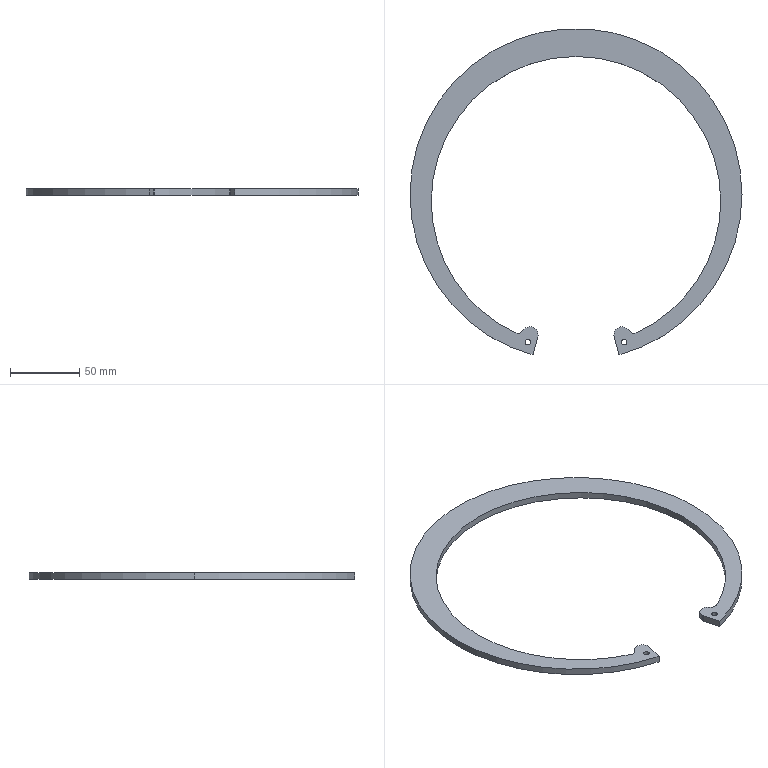Part | SolidWorks | features Extrusion 1 | 1 solid | 19 faces | box 240.5 x 236.403 x 4.75 mm | volume 49385 mm3 | cylinder 15 | plane 4 | commonest cylinder face diameters 4 x4 12 x3 209.7 x3 240.5 x3 8 x2
STEP:
#1=CARTESIAN_POINT('',(32.871,-106.959,2.375));
#2=VERTEX_POINT('',#1);
#3=CARTESIAN_POINT('',(36.871,-106.959,2.375));
#4=VERTEX_POINT('',#3);
#5=CARTESIAN_POINT('',(34.871,-106.959,2.375));
#6=DIRECTION('',(0.,0.,1.));
#7=DIRECTION('',(-1.,0.,0.));
#8=AXIS2_PLACEMENT_3D('',#5,#6,#7);
#9=CIRCLE('',#8,2.);
#10=EDGE_CURVE('',#2,#4,#9,.T.);
#11=ORIENTED_EDGE('',*,*,#10,.T.);
#12=CARTESIAN_POINT('',(36.871,-106.959,-2.375));
#13=VERTEX_POINT('',#12);
#14=CARTESIAN_POINT('',(36.871,-106.959,2.375));
#15=DIRECTION('',(0.,0.,-1.));
#16=VECTOR('',#15,1000.);
#17=LINE('',#14,#16);
#18=EDGE_CURVE('',#4,#13,#17,.T.);
#19=ORIENTED_EDGE('',*,*,#18,.T.);
#20=CARTESIAN_POINT('',(32.871,-106.959,-2.375));
#21=VERTEX_POINT('',#20);
#22=CARTESIAN_POINT('',(34.871,-106.959,-2.375));
#23=DIRECTION('',(0.,0.,1.));
#24=DIRECTION('',(-1.,0.,0.));
#25=AXIS2_PLACEMENT_3D('',#22,#23,#24);
#26=CIRCLE('',#25,2.);
#27=EDGE_CURVE('',#21,#13,#26,.T.);
#28=ORIENTED_EDGE('',*,*,#27,.F.);
#29=CARTESIAN_POINT('',(32.871,-106.959,2.375));
#30=DIRECTION('',(0.,0.,-1.));
#31=VECTOR('',#30,1000.);
#32=LINE('',#29,#31);
#33=EDGE_CURVE('',#2,#21,#32,.T.);
#34=ORIENTED_EDGE('',*,*,#33,.F.);
#35=EDGE_LOOP('',(#11,#19,#28,#34));
#36=FACE_OUTER_BOUND('',#35,.T.);
#37=CARTESIAN_POINT('',(34.871,-106.959,2.375));
#38=DIRECTION('',(0.,0.,-1.));
#39=DIRECTION('',(-1.,0.,0.));
#40=AXIS2_PLACEMENT_3D('',#37,#38,#39);
#41=CYLINDRICAL_SURFACE('',#40,2.);
#42=ADVANCED_FACE('',(#36),#41,.F.);
#43=CARTESIAN_POINT('',(-36.871,-106.959,2.375));
#44=VERTEX_POINT('',#43);
#45=CARTESIAN_POINT('',(-32.871,-106.959,2.375));
#46=VERTEX_POINT('',#45);
#47=CARTESIAN_POINT('',(-34.871,-106.959,2.375));
#48=DIRECTION('',(0.,0.,1.));
#49=DIRECTION('',(1.,0.,0.));
#50=AXIS2_PLACEMENT_3D('',#47,#48,#49);
#51=CIRCLE('',#50,2.);
#52=EDGE_CURVE('',#44,#46,#51,.T.);
#53=ORIENTED_EDGE('',*,*,#52,.T.);
#54=CARTESIAN_POINT('',(-32.871,-106.959,-2.375));
#55=VERTEX_POINT('',#54);
#56=CARTESIAN_POINT('',(-32.871,-106.959,2.375));
#57=DIRECTION('',(0.,0.,-1.));
#58=VECTOR('',#57,1000.);
#59=LINE('',#56,#58);
#60=EDGE_CURVE('',#46,#55,#59,.T.);
#61=ORIENTED_EDGE('',*,*,#60,.T.);
#62=CARTESIAN_POINT('',(-36.871,-106.959,-2.375));
#63=VERTEX_POINT('',#62);
#64=CARTESIAN_POINT('',(-34.871,-106.959,-2.375));
#65=DIRECTION('',(0.,0.,1.));
#66=DIRECTION('',(1.,0.,0.));
#67=AXIS2_PLACEMENT_3D('',#64,#65,#66);
#68=CIRCLE('',#67,2.);
#69=EDGE_CURVE('',#63,#55,#68,.T.);
#70=ORIENTED_EDGE('',*,*,#69,.F.);
#71=CARTESIAN_POINT('',(-36.871,-106.959,2.375));
#72=DIRECTION('',(0.,0.,-1.));
#73=VECTOR('',#72,1000.);
#74=LINE('',#71,#73);
#75=EDGE_CURVE('',#44,#63,#74,.T.);
#76=ORIENTED_EDGE('',*,*,#75,.F.);
#77=EDGE_LOOP('',(#53,#61,#70,#76));
#78=FACE_OUTER_BOUND('',#77,.T.);
#79=CARTESIAN_POINT('',(-34.871,-106.959,2.375));
#80=DIRECTION('',(0.,0.,-1.));
#81=DIRECTION('',(-1.,0.,0.));
#82=AXIS2_PLACEMENT_3D('',#79,#80,#81);
#83=CYLINDRICAL_SURFACE('',#82,2.);
#84=ADVANCED_FACE('',(#78),#83,.F.);
#85=CARTESIAN_POINT('',(120.25,0.,2.375));
#86=VERTEX_POINT('',#85);
#87=CARTESIAN_POINT('',(-120.25,0.,2.375));
#88=VERTEX_POINT('',#87);
#89=CARTESIAN_POINT('',(0.,0.,2.375));
#90=DIRECTION('',(0.,0.,1.));
#91=DIRECTION('',(1.,0.,0.));
#92=AXIS2_PLACEMENT_3D('',#89,#90,#91);
#93=CIRCLE('',#92,120.25);
#94=EDGE_CURVE('',#86,#88,#93,.T.);
#95=ORIENTED_EDGE('',*,*,#94,.F.);
#96=CARTESIAN_POINT('',(120.25,0.,-2.375));
#97=VERTEX_POINT('',#96);
#98=CARTESIAN_POINT('',(120.25,0.,2.375));
#99=DIRECTION('',(0.,0.,-1.));
#100=VECTOR('',#99,1000.);
#101=LINE('',#98,#100);
#102=EDGE_CURVE('',#86,#97,#101,.T.);
#103=ORIENTED_EDGE('',*,*,#102,.T.);
#104=CARTESIAN_POINT('',(-120.25,0.,-2.375));
#105=VERTEX_POINT('',#104);
#106=CARTESIAN_POINT('',(0.,0.,-2.375));
#107=DIRECTION('',(0.,0.,1.));
#108=DIRECTION('',(1.,0.,0.));
#109=AXIS2_PLACEMENT_3D('',#106,#107,#108);
#110=CIRCLE('',#109,120.25);
#111=EDGE_CURVE('',#97,#105,#110,.T.);
#112=ORIENTED_EDGE('',*,*,#111,.T.);
#113=CARTESIAN_POINT('',(-120.25,0.,2.375));
#114=DIRECTION('',(0.,0.,-1.));
#115=VECTOR('',#114,1000.);
#116=LINE('',#113,#115);
#117=EDGE_CURVE('',#88,#105,#116,.T.);
#118=ORIENTED_EDGE('',*,*,#117,.F.);
#119=EDGE_LOOP('',(#95,#103,#112,#118));
#120=FACE_OUTER_BOUND('',#119,.T.);
#121=CARTESIAN_POINT('',(0.,0.,2.375));
#122=DIRECTION('',(0.,0.,-1.));
#123=DIRECTION('',(-1.,0.,0.));
#124=AXIS2_PLACEMENT_3D('',#121,#122,#123);
#125=CYLINDRICAL_SURFACE('',#124,120.25);
#126=ADVANCED_FACE('',(#120),#125,.T.);
#127=CARTESIAN_POINT('',(-31.123,-116.153,2.375));
#128=VERTEX_POINT('',#127);
#129=CARTESIAN_POINT('',(0.,0.,2.375));
#130=DIRECTION('',(0.,0.,1.));
#131=DIRECTION('',(1.,0.,0.));
#132=AXIS2_PLACEMENT_3D('',#129,#130,#131);
#133=CIRCLE('',#132,120.25);
#134=EDGE_CURVE('',#88,#128,#133,.T.);
#135=ORIENTED_EDGE('',*,*,#134,.F.);
#136=ORIENTED_EDGE('',*,*,#117,.T.);
#137=CARTESIAN_POINT('',(-31.123,-116.153,-2.375));
#138=VERTEX_POINT('',#137);
#139=CARTESIAN_POINT('',(0.,0.,-2.375));
#140=DIRECTION('',(0.,0.,1.));
#141=DIRECTION('',(1.,0.,0.));
#142=AXIS2_PLACEMENT_3D('',#139,#140,#141);
#143=CIRCLE('',#142,120.25);
#144=EDGE_CURVE('',#105,#138,#143,.T.);
#145=ORIENTED_EDGE('',*,*,#144,.T.);
#146=CARTESIAN_POINT('',(-31.123,-116.153,2.375));
#147=DIRECTION('',(0.,0.,-1.));
#148=VECTOR('',#147,1000.);
#149=LINE('',#146,#148);
#150=EDGE_CURVE('',#128,#138,#149,.T.);
#151=ORIENTED_EDGE('',*,*,#150,.F.);
#152=EDGE_LOOP('',(#135,#136,#145,#151));
#153=FACE_OUTER_BOUND('',#152,.T.);
#154=CARTESIAN_POINT('',(0.,0.,2.375));
#155=DIRECTION('',(0.,0.,-1.));
#156=DIRECTION('',(-1.,0.,0.));
#157=AXIS2_PLACEMENT_3D('',#154,#155,#156);
#158=CYLINDRICAL_SURFACE('',#157,120.25);
#159=ADVANCED_FACE('',(#153),#158,.T.);
#160=CARTESIAN_POINT('',(27.485,-101.784,2.375));
#161=VERTEX_POINT('',#160);
#162=CARTESIAN_POINT('',(27.689,-103.337,2.375));
#163=VERTEX_POINT('',#162);
#164=CARTESIAN_POINT('',(33.485,-101.784,2.375));
#165=DIRECTION('',(0.,0.,1.));
#166=DIRECTION('',(-1.,0.,0.));
#167=AXIS2_PLACEMENT_3D('',#164,#165,#166);
#168=CIRCLE('',#167,6.);
#169=EDGE_CURVE('',#161,#163,#168,.T.);
#170=ORIENTED_EDGE('',*,*,#169,.F.);
#171=CARTESIAN_POINT('',(27.485,-101.784,-2.375));
#172=VERTEX_POINT('',#171);
#173=CARTESIAN_POINT('',(27.485,-101.784,2.375));
#174=DIRECTION('',(0.,0.,-1.));
#175=VECTOR('',#174,1000.);
#176=LINE('',#173,#175);
#177=EDGE_CURVE('',#161,#172,#176,.T.);
#178=ORIENTED_EDGE('',*,*,#177,.T.);
#179=CARTESIAN_POINT('',(27.689,-103.337,-2.375));
#180=VERTEX_POINT('',#179);
#181=CARTESIAN_POINT('',(33.485,-101.784,-2.375));
#182=DIRECTION('',(0.,0.,1.));
#183=DIRECTION('',(-1.,0.,0.));
#184=AXIS2_PLACEMENT_3D('',#181,#182,#183);
#185=CIRCLE('',#184,6.);
#186=EDGE_CURVE('',#172,#180,#185,.T.);
#187=ORIENTED_EDGE('',*,*,#186,.T.);
#188=CARTESIAN_POINT('',(27.689,-103.337,2.375));
#189=DIRECTION('',(0.,0.,-1.));
#190=VECTOR('',#189,1000.);
#191=LINE('',#188,#190);
#192=EDGE_CURVE('',#163,#180,#191,.T.);
#193=ORIENTED_EDGE('',*,*,#192,.F.);
#194=EDGE_LOOP('',(#170,#178,#187,#193));
#195=FACE_OUTER_BOUND('',#194,.T.);
#196=CARTESIAN_POINT('',(33.485,-101.784,2.375));
#197=DIRECTION('',(0.,0.,-1.));
#198=DIRECTION('',(-1.,0.,0.));
#199=AXIS2_PLACEMENT_3D('',#196,#197,#198);
#200=CYLINDRICAL_SURFACE('',#199,6.);
#201=ADVANCED_FACE('',(#195),#200,.T.);
#202=CARTESIAN_POINT('',(104.85,-4.8,2.375));
#203=VERTEX_POINT('',#202);
#204=CARTESIAN_POINT('',(43.639,-100.137,2.375));
#205=VERTEX_POINT('',#204);
#206=CARTESIAN_POINT('',(0.,-4.8,2.375));
#207=DIRECTION('',(0.,0.,-1.));
#208=DIRECTION('',(1.,0.,0.));
#209=AXIS2_PLACEMENT_3D('',#206,#207,#208);
#210=CIRCLE('',#209,104.85);
#211=EDGE_CURVE('',#203,#205,#210,.T.);
#212=ORIENTED_EDGE('',*,*,#211,.F.);
#213=CARTESIAN_POINT('',(104.85,-4.8,-2.375));
#214=VERTEX_POINT('',#213);
#215=CARTESIAN_POINT('',(104.85,-4.8,2.375));
#216=DIRECTION('',(0.,0.,-1.));
#217=VECTOR('',#216,1000.);
#218=LINE('',#215,#217);
#219=EDGE_CURVE('',#203,#214,#218,.T.);
#220=ORIENTED_EDGE('',*,*,#219,.T.);
#221=CARTESIAN_POINT('',(43.639,-100.137,-2.375));
#222=VERTEX_POINT('',#221);
#223=CARTESIAN_POINT('',(0.,-4.8,-2.375));
#224=DIRECTION('',(0.,0.,-1.));
#225=DIRECTION('',(1.,0.,0.));
#226=AXIS2_PLACEMENT_3D('',#223,#224,#225);
#227=CIRCLE('',#226,104.85);
#228=EDGE_CURVE('',#214,#222,#227,.T.);
#229=ORIENTED_EDGE('',*,*,#228,.T.);
#230=CARTESIAN_POINT('',(43.639,-100.137,2.375));
#231=DIRECTION('',(0.,0.,-1.));
#232=VECTOR('',#231,1000.);
#233=LINE('',#230,#232);
#234=EDGE_CURVE('',#205,#222,#233,.T.);
#235=ORIENTED_EDGE('',*,*,#234,.F.);
#236=EDGE_LOOP('',(#212,#220,#229,#235));
#237=FACE_OUTER_BOUND('',#236,.T.);
#238=CARTESIAN_POINT('',(0.,-4.8,2.375));
#239=DIRECTION('',(0.,0.,-1.));
#240=DIRECTION('',(-1.,0.,0.));
#241=AXIS2_PLACEMENT_3D('',#238,#239,#240);
#242=CYLINDRICAL_SURFACE('',#241,104.85);
#243=ADVANCED_FACE('',(#237),#242,.F.);
#244=ORIENTED_EDGE('',*,*,#219,.F.);
#245=CARTESIAN_POINT('',(-104.85,-4.8,2.375));
#246=VERTEX_POINT('',#245);
#247=CARTESIAN_POINT('',(0.,-4.8,2.375));
#248=DIRECTION('',(0.,0.,-1.));
#249=DIRECTION('',(1.,0.,0.));
#250=AXIS2_PLACEMENT_3D('',#247,#248,#249);
#251=CIRCLE('',#250,104.85);
#252=EDGE_CURVE('',#246,#203,#251,.T.);
#253=ORIENTED_EDGE('',*,*,#252,.F.);
#254=CARTESIAN_POINT('',(-104.85,-4.8,-2.375));
#255=VERTEX_POINT('',#254);
#256=CARTESIAN_POINT('',(-104.85,-4.8,2.375));
#257=DIRECTION('',(0.,0.,-1.));
#258=VECTOR('',#257,1000.);
#259=LINE('',#256,#258);
#260=EDGE_CURVE('',#246,#255,#259,.T.);
#261=ORIENTED_EDGE('',*,*,#260,.T.);
#262=CARTESIAN_POINT('',(0.,-4.8,-2.375));
#263=DIRECTION('',(0.,0.,-1.));
#264=DIRECTION('',(1.,0.,0.));
#265=AXIS2_PLACEMENT_3D('',#262,#263,#264);
#266=CIRCLE('',#265,104.85);
#267=EDGE_CURVE('',#255,#214,#266,.T.);
#268=ORIENTED_EDGE('',*,*,#267,.T.);
#269=EDGE_LOOP('',(#244,#253,#261,#268));
#270=FACE_OUTER_BOUND('',#269,.T.);
#271=CARTESIAN_POINT('',(0.,-4.8,2.375));
#272=DIRECTION('',(0.,0.,-1.));
#273=DIRECTION('',(-1.,0.,0.));
#274=AXIS2_PLACEMENT_3D('',#271,#272,#273);
#275=CYLINDRICAL_SURFACE('',#274,104.85);
#276=ADVANCED_FACE('',(#270),#275,.F.);
#277=ORIENTED_EDGE('',*,*,#52,.F.);
#278=CARTESIAN_POINT('',(-34.871,-106.959,2.375));
#279=DIRECTION('',(0.,0.,1.));
#280=DIRECTION('',(1.,0.,0.));
#281=AXIS2_PLACEMENT_3D('',#278,#279,#280);
#282=CIRCLE('',#281,2.);
#283=EDGE_CURVE('',#46,#44,#282,.T.);
#284=ORIENTED_EDGE('',*,*,#283,.F.);
#285=EDGE_LOOP('',(#277,#284));
#286=FACE_BOUND('',#285,.T.);
#287=CARTESIAN_POINT('',(-27.689,-103.337,2.375));
#288=VERTEX_POINT('',#287);
#289=CARTESIAN_POINT('',(-38.579,-98.613,2.375));
#290=VERTEX_POINT('',#289);
#291=CARTESIAN_POINT('',(-33.485,-101.784,2.375));
#292=DIRECTION('',(0.,0.,1.));
#293=DIRECTION('',(1.,0.,0.));
#294=AXIS2_PLACEMENT_3D('',#291,#292,#293);
#295=CIRCLE('',#294,6.);
#296=EDGE_CURVE('',#288,#290,#295,.T.);
#297=ORIENTED_EDGE('',*,*,#296,.T.);
#298=CARTESIAN_POINT('',(-43.639,-100.137,2.375));
#299=VERTEX_POINT('',#298);
#300=CARTESIAN_POINT('',(-41.975,-96.5,2.375));
#301=DIRECTION('',(0.,0.,-1.));
#302=DIRECTION('',(-1.,0.,0.));
#303=AXIS2_PLACEMENT_3D('',#300,#301,#302);
#304=CIRCLE('',#303,4.);
#305=EDGE_CURVE('',#290,#299,#304,.T.);
#306=ORIENTED_EDGE('',*,*,#305,.T.);
#307=CARTESIAN_POINT('',(0.,-4.8,2.375));
#308=DIRECTION('',(0.,0.,-1.));
#309=DIRECTION('',(1.,0.,0.));
#310=AXIS2_PLACEMENT_3D('',#307,#308,#309);
#311=CIRCLE('',#310,104.85);
#312=EDGE_CURVE('',#299,#246,#311,.T.);
#313=ORIENTED_EDGE('',*,*,#312,.T.);
#314=ORIENTED_EDGE('',*,*,#252,.T.);
#315=ORIENTED_EDGE('',*,*,#211,.T.);
#316=CARTESIAN_POINT('',(38.579,-98.613,2.375));
#317=VERTEX_POINT('',#316);
#318=CARTESIAN_POINT('',(41.975,-96.5,2.375));
#319=DIRECTION('',(0.,0.,-1.));
#320=DIRECTION('',(1.,0.,0.));
#321=AXIS2_PLACEMENT_3D('',#318,#319,#320);
#322=CIRCLE('',#321,4.);
#323=EDGE_CURVE('',#205,#317,#322,.T.);
#324=ORIENTED_EDGE('',*,*,#323,.T.);
#325=CARTESIAN_POINT('',(33.485,-101.784,2.375));
#326=DIRECTION('',(0.,0.,1.));
#327=DIRECTION('',(-1.,0.,0.));
#328=AXIS2_PLACEMENT_3D('',#325,#326,#327);
#329=CIRCLE('',#328,6.);
#330=EDGE_CURVE('',#317,#161,#329,.T.);
#331=ORIENTED_EDGE('',*,*,#330,.T.);
#332=ORIENTED_EDGE('',*,*,#169,.T.);
#333=CARTESIAN_POINT('',(31.123,-116.153,2.375));
#334=VERTEX_POINT('',#333);
#335=CARTESIAN_POINT('',(27.689,-103.337,2.375));
#336=DIRECTION('',(0.2588,-0.9659,0.));
#337=VECTOR('',#336,1000.);
#338=LINE('',#335,#337);
#339=EDGE_CURVE('',#163,#334,#338,.T.);
#340=ORIENTED_EDGE('',*,*,#339,.T.);
#341=CARTESIAN_POINT('',(0.,0.,2.375));
#342=DIRECTION('',(0.,0.,1.));
#343=DIRECTION('',(1.,0.,0.));
#344=AXIS2_PLACEMENT_3D('',#341,#342,#343);
#345=CIRCLE('',#344,120.25);
#346=EDGE_CURVE('',#334,#86,#345,.T.);
#347=ORIENTED_EDGE('',*,*,#346,.T.);
#348=ORIENTED_EDGE('',*,*,#94,.T.);
#349=ORIENTED_EDGE('',*,*,#134,.T.);
#350=CARTESIAN_POINT('',(-27.689,-103.337,2.375));
#351=DIRECTION('',(0.2588,0.9659,0.));
#352=VECTOR('',#351,1000.);
#353=LINE('',#350,#352);
#354=EDGE_CURVE('',#128,#288,#353,.T.);
#355=ORIENTED_EDGE('',*,*,#354,.T.);
#356=EDGE_LOOP('',(#297,#306,#313,#314,#315,#324,#331,#332,#340,#347,#348,#349,#355));
#357=FACE_OUTER_BOUND('',#356,.T.);
#358=ORIENTED_EDGE('',*,*,#10,.F.);
#359=CARTESIAN_POINT('',(34.871,-106.959,2.375));
#360=DIRECTION('',(0.,0.,1.));
#361=DIRECTION('',(-1.,0.,0.));
#362=AXIS2_PLACEMENT_3D('',#359,#360,#361);
#363=CIRCLE('',#362,2.);
#364=EDGE_CURVE('',#4,#2,#363,.T.);
#365=ORIENTED_EDGE('',*,*,#364,.F.);
#366=EDGE_LOOP('',(#358,#365));
#367=FACE_BOUND('',#366,.T.);
#368=CARTESIAN_POINT('',(-33.485,-101.784,2.375));
#369=DIRECTION('',(0.,0.,1.));
#370=DIRECTION('',(1.,0.,0.));
#371=AXIS2_PLACEMENT_3D('',#368,#369,#370);
#372=PLANE('',#371);
#373=ADVANCED_FACE('',(#286,#357,#367),#372,.T.);
#374=ORIENTED_EDGE('',*,*,#69,.T.);
#375=CARTESIAN_POINT('',(-34.871,-106.959,-2.375));
#376=DIRECTION('',(0.,0.,1.));
#377=DIRECTION('',(1.,0.,0.));
#378=AXIS2_PLACEMENT_3D('',#375,#376,#377);
#379=CIRCLE('',#378,2.);
#380=EDGE_CURVE('',#55,#63,#379,.T.);
#381=ORIENTED_EDGE('',*,*,#380,.T.);
#382=EDGE_LOOP('',(#374,#381));
#383=FACE_BOUND('',#382,.T.);
#384=CARTESIAN_POINT('',(-27.689,-103.337,-2.375));
#385=VERTEX_POINT('',#384);
#386=CARTESIAN_POINT('',(-38.579,-98.613,-2.375));
#387=VERTEX_POINT('',#386);
#388=CARTESIAN_POINT('',(-33.485,-101.784,-2.375));
#389=DIRECTION('',(0.,0.,1.));
#390=DIRECTION('',(1.,0.,0.));
#391=AXIS2_PLACEMENT_3D('',#388,#389,#390);
#392=CIRCLE('',#391,6.);
#393=EDGE_CURVE('',#385,#387,#392,.T.);
#394=ORIENTED_EDGE('',*,*,#393,.F.);
#395=CARTESIAN_POINT('',(-27.689,-103.337,-2.375));
#396=DIRECTION('',(0.2588,0.9659,0.));
#397=VECTOR('',#396,1000.);
#398=LINE('',#395,#397);
#399=EDGE_CURVE('',#138,#385,#398,.T.);
#400=ORIENTED_EDGE('',*,*,#399,.F.);
#401=ORIENTED_EDGE('',*,*,#144,.F.);
#402=ORIENTED_EDGE('',*,*,#111,.F.);
#403=CARTESIAN_POINT('',(31.123,-116.153,-2.375));
#404=VERTEX_POINT('',#403);
#405=CARTESIAN_POINT('',(0.,0.,-2.375));
#406=DIRECTION('',(0.,0.,1.));
#407=DIRECTION('',(1.,0.,0.));
#408=AXIS2_PLACEMENT_3D('',#405,#406,#407);
#409=CIRCLE('',#408,120.25);
#410=EDGE_CURVE('',#404,#97,#409,.T.);
#411=ORIENTED_EDGE('',*,*,#410,.F.);
#412=CARTESIAN_POINT('',(27.689,-103.337,-2.375));
#413=DIRECTION('',(0.2588,-0.9659,0.));
#414=VECTOR('',#413,1000.);
#415=LINE('',#412,#414);
#416=EDGE_CURVE('',#180,#404,#415,.T.);
#417=ORIENTED_EDGE('',*,*,#416,.F.);
#418=ORIENTED_EDGE('',*,*,#186,.F.);
#419=CARTESIAN_POINT('',(38.579,-98.613,-2.375));
#420=VERTEX_POINT('',#419);
#421=CARTESIAN_POINT('',(33.485,-101.784,-2.375));
#422=DIRECTION('',(0.,0.,1.));
#423=DIRECTION('',(-1.,0.,0.));
#424=AXIS2_PLACEMENT_3D('',#421,#422,#423);
#425=CIRCLE('',#424,6.);
#426=EDGE_CURVE('',#420,#172,#425,.T.);
#427=ORIENTED_EDGE('',*,*,#426,.F.);
#428=CARTESIAN_POINT('',(41.975,-96.5,-2.375));
#429=DIRECTION('',(0.,0.,-1.));
#430=DIRECTION('',(1.,0.,0.));
#431=AXIS2_PLACEMENT_3D('',#428,#429,#430);
#432=CIRCLE('',#431,4.);
#433=EDGE_CURVE('',#222,#420,#432,.T.);
#434=ORIENTED_EDGE('',*,*,#433,.F.);
#435=ORIENTED_EDGE('',*,*,#228,.F.);
#436=ORIENTED_EDGE('',*,*,#267,.F.);
#437=CARTESIAN_POINT('',(-43.639,-100.137,-2.375));
#438=VERTEX_POINT('',#437);
#439=CARTESIAN_POINT('',(0.,-4.8,-2.375));
#440=DIRECTION('',(0.,0.,-1.));
#441=DIRECTION('',(1.,0.,0.));
#442=AXIS2_PLACEMENT_3D('',#439,#440,#441);
#443=CIRCLE('',#442,104.85);
#444=EDGE_CURVE('',#438,#255,#443,.T.);
#445=ORIENTED_EDGE('',*,*,#444,.F.);
#446=CARTESIAN_POINT('',(-41.975,-96.5,-2.375));
#447=DIRECTION('',(0.,0.,-1.));
#448=DIRECTION('',(-1.,0.,0.));
#449=AXIS2_PLACEMENT_3D('',#446,#447,#448);
#450=CIRCLE('',#449,4.);
#451=EDGE_CURVE('',#387,#438,#450,.T.);
#452=ORIENTED_EDGE('',*,*,#451,.F.);
#453=EDGE_LOOP('',(#394,#400,#401,#402,#411,#417,#418,#427,#434,#435,#436,#445,#452));
#454=FACE_OUTER_BOUND('',#453,.T.);
#455=ORIENTED_EDGE('',*,*,#27,.T.);
#456=CARTESIAN_POINT('',(34.871,-106.959,-2.375));
#457=DIRECTION('',(0.,0.,1.));
#458=DIRECTION('',(-1.,0.,0.));
#459=AXIS2_PLACEMENT_3D('',#456,#457,#458);
#460=CIRCLE('',#459,2.);
#461=EDGE_CURVE('',#13,#21,#460,.T.);
#462=ORIENTED_EDGE('',*,*,#461,.T.);
#463=EDGE_LOOP('',(#455,#462));
#464=FACE_BOUND('',#463,.T.);
#465=CARTESIAN_POINT('',(-33.485,-101.784,-2.375));
#466=DIRECTION('',(0.,0.,1.));
#467=DIRECTION('',(1.,0.,0.));
#468=AXIS2_PLACEMENT_3D('',#465,#466,#467);
#469=PLANE('',#468);
#470=ADVANCED_FACE('',(#383,#454,#464),#469,.F.);
#471=ORIENTED_EDGE('',*,*,#393,.T.);
#472=CARTESIAN_POINT('',(-38.579,-98.613,2.375));
#473=DIRECTION('',(0.,0.,-1.));
#474=VECTOR('',#473,1000.);
#475=LINE('',#472,#474);
#476=EDGE_CURVE('',#290,#387,#475,.T.);
#477=ORIENTED_EDGE('',*,*,#476,.F.);
#478=ORIENTED_EDGE('',*,*,#296,.F.);
#479=CARTESIAN_POINT('',(-27.689,-103.337,2.375));
#480=DIRECTION('',(0.,0.,-1.));
#481=VECTOR('',#480,1000.);
#482=LINE('',#479,#481);
#483=EDGE_CURVE('',#288,#385,#482,.T.);
#484=ORIENTED_EDGE('',*,*,#483,.T.);
#485=EDGE_LOOP('',(#471,#477,#478,#484));
#486=FACE_OUTER_BOUND('',#485,.T.);
#487=CARTESIAN_POINT('',(-33.485,-101.784,2.375));
#488=DIRECTION('',(0.,0.,-1.));
#489=DIRECTION('',(-1.,0.,0.));
#490=AXIS2_PLACEMENT_3D('',#487,#488,#489);
#491=CYLINDRICAL_SURFACE('',#490,6.);
#492=ADVANCED_FACE('',(#486),#491,.T.);
#493=ORIENTED_EDGE('',*,*,#451,.T.);
#494=CARTESIAN_POINT('',(-43.639,-100.137,2.375));
#495=DIRECTION('',(0.,0.,-1.));
#496=VECTOR('',#495,1000.);
#497=LINE('',#494,#496);
#498=EDGE_CURVE('',#299,#438,#497,.T.);
#499=ORIENTED_EDGE('',*,*,#498,.F.);
#500=ORIENTED_EDGE('',*,*,#305,.F.);
#501=ORIENTED_EDGE('',*,*,#476,.T.);
#502=EDGE_LOOP('',(#493,#499,#500,#501));
#503=FACE_OUTER_BOUND('',#502,.T.);
#504=CARTESIAN_POINT('',(-41.975,-96.5,2.375));
#505=DIRECTION('',(0.,0.,-1.));
#506=DIRECTION('',(-1.,0.,0.));
#507=AXIS2_PLACEMENT_3D('',#504,#505,#506);
#508=CYLINDRICAL_SURFACE('',#507,4.);
#509=ADVANCED_FACE('',(#503),#508,.F.);
#510=ORIENTED_EDGE('',*,*,#260,.F.);
#511=ORIENTED_EDGE('',*,*,#312,.F.);
#512=ORIENTED_EDGE('',*,*,#498,.T.);
#513=ORIENTED_EDGE('',*,*,#444,.T.);
#514=EDGE_LOOP('',(#510,#511,#512,#513));
#515=FACE_OUTER_BOUND('',#514,.T.);
#516=CARTESIAN_POINT('',(0.,-4.8,2.375));
#517=DIRECTION('',(0.,0.,-1.));
#518=DIRECTION('',(-1.,0.,0.));
#519=AXIS2_PLACEMENT_3D('',#516,#517,#518);
#520=CYLINDRICAL_SURFACE('',#519,104.85);
#521=ADVANCED_FACE('',(#515),#520,.F.);
#522=ORIENTED_EDGE('',*,*,#433,.T.);
#523=CARTESIAN_POINT('',(38.579,-98.613,2.375));
#524=DIRECTION('',(0.,0.,-1.));
#525=VECTOR('',#524,1000.);
#526=LINE('',#523,#525);
#527=EDGE_CURVE('',#317,#420,#526,.T.);
#528=ORIENTED_EDGE('',*,*,#527,.F.);
#529=ORIENTED_EDGE('',*,*,#323,.F.);
#530=ORIENTED_EDGE('',*,*,#234,.T.);
#531=EDGE_LOOP('',(#522,#528,#529,#530));
#532=FACE_OUTER_BOUND('',#531,.T.);
#533=CARTESIAN_POINT('',(41.975,-96.5,2.375));
#534=DIRECTION('',(0.,0.,-1.));
#535=DIRECTION('',(-1.,0.,0.));
#536=AXIS2_PLACEMENT_3D('',#533,#534,#535);
#537=CYLINDRICAL_SURFACE('',#536,4.);
#538=ADVANCED_FACE('',(#532),#537,.F.);
#539=ORIENTED_EDGE('',*,*,#177,.F.);
#540=ORIENTED_EDGE('',*,*,#330,.F.);
#541=ORIENTED_EDGE('',*,*,#527,.T.);
#542=ORIENTED_EDGE('',*,*,#426,.T.);
#543=EDGE_LOOP('',(#539,#540,#541,#542));
#544=FACE_OUTER_BOUND('',#543,.T.);
#545=CARTESIAN_POINT('',(33.485,-101.784,2.375));
#546=DIRECTION('',(0.,0.,-1.));
#547=DIRECTION('',(-1.,0.,0.));
#548=AXIS2_PLACEMENT_3D('',#545,#546,#547);
#549=CYLINDRICAL_SURFACE('',#548,6.);
#550=ADVANCED_FACE('',(#544),#549,.T.);
#551=ORIENTED_EDGE('',*,*,#416,.T.);
#552=CARTESIAN_POINT('',(31.123,-116.153,2.375));
#553=DIRECTION('',(0.,0.,-1.));
#554=VECTOR('',#553,1000.);
#555=LINE('',#552,#554);
#556=EDGE_CURVE('',#334,#404,#555,.T.);
#557=ORIENTED_EDGE('',*,*,#556,.F.);
#558=ORIENTED_EDGE('',*,*,#339,.F.);
#559=ORIENTED_EDGE('',*,*,#192,.T.);
#560=EDGE_LOOP('',(#551,#557,#558,#559));
#561=FACE_OUTER_BOUND('',#560,.T.);
#562=CARTESIAN_POINT('',(27.689,-103.337,2.375));
#563=DIRECTION('',(0.9659,0.2588,0.));
#564=DIRECTION('',(-0.2588,0.9659,0.));
#565=AXIS2_PLACEMENT_3D('',#562,#563,#564);
#566=PLANE('',#565);
#567=ADVANCED_FACE('',(#561),#566,.F.);
#568=ORIENTED_EDGE('',*,*,#102,.F.);
#569=ORIENTED_EDGE('',*,*,#346,.F.);
#570=ORIENTED_EDGE('',*,*,#556,.T.);
#571=ORIENTED_EDGE('',*,*,#410,.T.);
#572=EDGE_LOOP('',(#568,#569,#570,#571));
#573=FACE_OUTER_BOUND('',#572,.T.);
#574=CARTESIAN_POINT('',(0.,0.,2.375));
#575=DIRECTION('',(0.,0.,-1.));
#576=DIRECTION('',(-1.,0.,0.));
#577=AXIS2_PLACEMENT_3D('',#574,#575,#576);
#578=CYLINDRICAL_SURFACE('',#577,120.25);
#579=ADVANCED_FACE('',(#573),#578,.T.);
#580=ORIENTED_EDGE('',*,*,#399,.T.);
#581=ORIENTED_EDGE('',*,*,#483,.F.);
#582=ORIENTED_EDGE('',*,*,#354,.F.);
#583=ORIENTED_EDGE('',*,*,#150,.T.);
#584=EDGE_LOOP('',(#580,#581,#582,#583));
#585=FACE_OUTER_BOUND('',#584,.T.);
#586=CARTESIAN_POINT('',(-27.689,-103.337,2.375));
#587=DIRECTION('',(-0.9659,0.2588,0.));
#588=DIRECTION('',(-0.2588,-0.9659,0.));
#589=AXIS2_PLACEMENT_3D('',#586,#587,#588);
#590=PLANE('',#589);
#591=ADVANCED_FACE('',(#585),#590,.F.);
#592=ORIENTED_EDGE('',*,*,#60,.F.);
#593=ORIENTED_EDGE('',*,*,#283,.T.);
#594=ORIENTED_EDGE('',*,*,#75,.T.);
#595=ORIENTED_EDGE('',*,*,#380,.F.);
#596=EDGE_LOOP('',(#592,#593,#594,#595));
#597=FACE_OUTER_BOUND('',#596,.T.);
#598=CARTESIAN_POINT('',(-34.871,-106.959,2.375));
#599=DIRECTION('',(0.,0.,-1.));
#600=DIRECTION('',(-1.,0.,0.));
#601=AXIS2_PLACEMENT_3D('',#598,#599,#600);
#602=CYLINDRICAL_SURFACE('',#601,2.);
#603=ADVANCED_FACE('',(#597),#602,.F.);
#604=ORIENTED_EDGE('',*,*,#18,.F.);
#605=ORIENTED_EDGE('',*,*,#364,.T.);
#606=ORIENTED_EDGE('',*,*,#33,.T.);
#607=ORIENTED_EDGE('',*,*,#461,.F.);
#608=EDGE_LOOP('',(#604,#605,#606,#607));
#609=FACE_OUTER_BOUND('',#608,.T.);
#610=CARTESIAN_POINT('',(34.871,-106.959,2.375));
#611=DIRECTION('',(0.,0.,-1.));
#612=DIRECTION('',(-1.,0.,0.));
#613=AXIS2_PLACEMENT_3D('',#610,#611,#612);
#614=CYLINDRICAL_SURFACE('',#613,2.);
#615=ADVANCED_FACE('',(#609),#614,.F.);
#616=CLOSED_SHELL('',(#42,#84,#126,#159,#201,#243,#276,#373,#470,#492,#509,#521,#538,#550,#567,#579,#591,#603,#615));
#617=MANIFOLD_SOLID_BREP('',#616);
#618=CARTESIAN_POINT('',(0.,0.,0.));
#619=DIRECTION('',(0.,0.,1.));
#620=DIRECTION('',(1.,0.,0.));
#621=AXIS2_PLACEMENT_3D('',#618,#619,#620);
#622=(LENGTH_UNIT()NAMED_UNIT(*)SI_UNIT(.MILLI.,.METRE.));
#623=UNCERTAINTY_MEASURE_WITH_UNIT(LENGTH_MEASURE(0.00001),#622,'','');
#624=(NAMED_UNIT(*)PLANE_ANGLE_UNIT()SI_UNIT($,.RADIAN.));
#625=(NAMED_UNIT(*)SI_UNIT($,.STERADIAN.)SOLID_ANGLE_UNIT());
#626=(GEOMETRIC_REPRESENTATION_CONTEXT(3)GLOBAL_UNCERTAINTY_ASSIGNED_CONTEXT((#623))GLOBAL_UNIT_ASSIGNED_CONTEXT((#622,#624,#625))REPRESENTATION_CONTEXT('',''));
#627=ADVANCED_BREP_SHAPE_REPRESENTATION('',(#617,#621),#626);